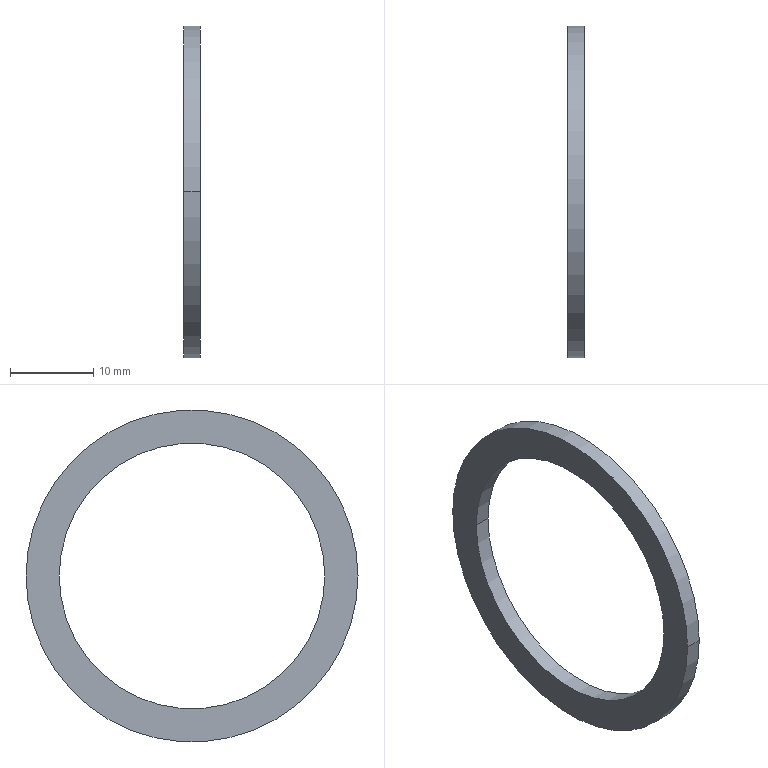Part | NX | features BREP 1 | 1 solid | 6 faces | box 2 x 40 x 40 mm | volume 904.779 mm3 | cylinder 4 | plane 2 | commonest cylinder face diameters 32 x2 40 x2
STEP:
#1=CARTESIAN_POINT('',(-531.355,16.,0.));
#2=VERTEX_POINT('',#1);
#3=CARTESIAN_POINT('',(-531.355,-16.,0.));
#4=VERTEX_POINT('',#3);
#5=CARTESIAN_POINT('',(-531.355,0.,0.));
#6=DIRECTION('',(-1.,0.,0.));
#7=DIRECTION('',(0.,-1.,0.));
#8=AXIS2_PLACEMENT_3D('',#5,#6,#7);
#9=CIRCLE('',#8,16.);
#10=EDGE_CURVE('',#2,#4,#9,.T.);
#11=ORIENTED_EDGE('',*,*,#10,.T.);
#12=CARTESIAN_POINT('',(-529.355,-16.,0.));
#13=VERTEX_POINT('',#12);
#14=CARTESIAN_POINT('',(-531.355,-16.,0.));
#15=DIRECTION('',(1.,0.,0.));
#16=VECTOR('',#15,1000.);
#17=LINE('',#14,#16);
#18=EDGE_CURVE('',#4,#13,#17,.T.);
#19=ORIENTED_EDGE('',*,*,#18,.T.);
#20=CARTESIAN_POINT('',(-529.355,16.,0.));
#21=VERTEX_POINT('',#20);
#22=CARTESIAN_POINT('',(-529.355,0.,0.));
#23=DIRECTION('',(-1.,0.,0.));
#24=DIRECTION('',(0.,-1.,0.));
#25=AXIS2_PLACEMENT_3D('',#22,#23,#24);
#26=CIRCLE('',#25,16.);
#27=EDGE_CURVE('',#21,#13,#26,.T.);
#28=ORIENTED_EDGE('',*,*,#27,.F.);
#29=CARTESIAN_POINT('',(-531.355,16.,0.));
#30=DIRECTION('',(1.,0.,0.));
#31=VECTOR('',#30,1000.);
#32=LINE('',#29,#31);
#33=EDGE_CURVE('',#2,#21,#32,.T.);
#34=ORIENTED_EDGE('',*,*,#33,.F.);
#35=EDGE_LOOP('',(#11,#19,#28,#34));
#36=FACE_BOUND('',#35,.T.);
#37=CARTESIAN_POINT('',(-531.355,0.,0.));
#38=DIRECTION('',(1.,0.,0.));
#39=DIRECTION('',(0.,1.,0.));
#40=AXIS2_PLACEMENT_3D('',#37,#38,#39);
#41=CYLINDRICAL_SURFACE('',#40,16.);
#42=ADVANCED_FACE('',(#36),#41,.F.);
#43=CARTESIAN_POINT('',(-531.355,-20.,0.));
#44=VERTEX_POINT('',#43);
#45=CARTESIAN_POINT('',(-531.355,20.,0.));
#46=VERTEX_POINT('',#45);
#47=CARTESIAN_POINT('',(-531.355,0.,0.));
#48=DIRECTION('',(-1.,0.,0.));
#49=DIRECTION('',(0.,-1.,0.));
#50=AXIS2_PLACEMENT_3D('',#47,#48,#49);
#51=CIRCLE('',#50,20.);
#52=EDGE_CURVE('',#44,#46,#51,.T.);
#53=ORIENTED_EDGE('',*,*,#52,.F.);
#54=CARTESIAN_POINT('',(-529.355,-20.,0.));
#55=VERTEX_POINT('',#54);
#56=CARTESIAN_POINT('',(-531.355,-20.,0.));
#57=DIRECTION('',(1.,0.,0.));
#58=VECTOR('',#57,1000.);
#59=LINE('',#56,#58);
#60=EDGE_CURVE('',#44,#55,#59,.T.);
#61=ORIENTED_EDGE('',*,*,#60,.T.);
#62=CARTESIAN_POINT('',(-529.355,20.,0.));
#63=VERTEX_POINT('',#62);
#64=CARTESIAN_POINT('',(-529.355,0.,0.));
#65=DIRECTION('',(-1.,0.,0.));
#66=DIRECTION('',(0.,-1.,0.));
#67=AXIS2_PLACEMENT_3D('',#64,#65,#66);
#68=CIRCLE('',#67,20.);
#69=EDGE_CURVE('',#55,#63,#68,.T.);
#70=ORIENTED_EDGE('',*,*,#69,.T.);
#71=CARTESIAN_POINT('',(-531.355,20.,0.));
#72=DIRECTION('',(1.,0.,0.));
#73=VECTOR('',#72,1000.);
#74=LINE('',#71,#73);
#75=EDGE_CURVE('',#46,#63,#74,.T.);
#76=ORIENTED_EDGE('',*,*,#75,.F.);
#77=EDGE_LOOP('',(#53,#61,#70,#76));
#78=FACE_BOUND('',#77,.T.);
#79=CARTESIAN_POINT('',(-531.355,0.,0.));
#80=DIRECTION('',(1.,0.,0.));
#81=DIRECTION('',(0.,1.,0.));
#82=AXIS2_PLACEMENT_3D('',#79,#80,#81);
#83=CYLINDRICAL_SURFACE('',#82,20.);
#84=ADVANCED_FACE('',(#78),#83,.T.);
#85=CARTESIAN_POINT('',(-531.355,0.,0.));
#86=DIRECTION('',(-1.,0.,0.));
#87=DIRECTION('',(0.,-1.,0.));
#88=AXIS2_PLACEMENT_3D('',#85,#86,#87);
#89=CIRCLE('',#88,20.);
#90=EDGE_CURVE('',#46,#44,#89,.T.);
#91=ORIENTED_EDGE('',*,*,#90,.T.);
#92=ORIENTED_EDGE('',*,*,#52,.T.);
#93=EDGE_LOOP('',(#91,#92));
#94=FACE_BOUND('',#93,.T.);
#95=ORIENTED_EDGE('',*,*,#10,.F.);
#96=CARTESIAN_POINT('',(-531.355,0.,0.));
#97=DIRECTION('',(-1.,0.,0.));
#98=DIRECTION('',(0.,-1.,0.));
#99=AXIS2_PLACEMENT_3D('',#96,#97,#98);
#100=CIRCLE('',#99,16.);
#101=EDGE_CURVE('',#4,#2,#100,.T.);
#102=ORIENTED_EDGE('',*,*,#101,.F.);
#103=EDGE_LOOP('',(#95,#102));
#104=FACE_BOUND('',#103,.T.);
#105=CARTESIAN_POINT('',(-531.355,0.,0.));
#106=DIRECTION('',(-1.,0.,0.));
#107=DIRECTION('',(0.,-1.,0.));
#108=AXIS2_PLACEMENT_3D('',#105,#106,#107);
#109=PLANE('',#108);
#110=ADVANCED_FACE('',(#94,#104),#109,.T.);
#111=CARTESIAN_POINT('',(-529.355,0.,0.));
#112=DIRECTION('',(-1.,0.,0.));
#113=DIRECTION('',(0.,-1.,0.));
#114=AXIS2_PLACEMENT_3D('',#111,#112,#113);
#115=CIRCLE('',#114,20.);
#116=EDGE_CURVE('',#63,#55,#115,.T.);
#117=ORIENTED_EDGE('',*,*,#116,.F.);
#118=ORIENTED_EDGE('',*,*,#69,.F.);
#119=EDGE_LOOP('',(#117,#118));
#120=FACE_BOUND('',#119,.T.);
#121=ORIENTED_EDGE('',*,*,#27,.T.);
#122=CARTESIAN_POINT('',(-529.355,0.,0.));
#123=DIRECTION('',(-1.,0.,0.));
#124=DIRECTION('',(0.,-1.,0.));
#125=AXIS2_PLACEMENT_3D('',#122,#123,#124);
#126=CIRCLE('',#125,16.);
#127=EDGE_CURVE('',#13,#21,#126,.T.);
#128=ORIENTED_EDGE('',*,*,#127,.T.);
#129=EDGE_LOOP('',(#121,#128));
#130=FACE_BOUND('',#129,.T.);
#131=CARTESIAN_POINT('',(-529.355,0.,0.));
#132=DIRECTION('',(-1.,0.,0.));
#133=DIRECTION('',(0.,-1.,0.));
#134=AXIS2_PLACEMENT_3D('',#131,#132,#133);
#135=PLANE('',#134);
#136=ADVANCED_FACE('',(#120,#130),#135,.F.);
#137=ORIENTED_EDGE('',*,*,#60,.F.);
#138=ORIENTED_EDGE('',*,*,#90,.F.);
#139=ORIENTED_EDGE('',*,*,#75,.T.);
#140=ORIENTED_EDGE('',*,*,#116,.T.);
#141=EDGE_LOOP('',(#137,#138,#139,#140));
#142=FACE_BOUND('',#141,.T.);
#143=CARTESIAN_POINT('',(-531.355,0.,0.));
#144=DIRECTION('',(1.,0.,0.));
#145=DIRECTION('',(0.,1.,0.));
#146=AXIS2_PLACEMENT_3D('',#143,#144,#145);
#147=CYLINDRICAL_SURFACE('',#146,20.);
#148=ADVANCED_FACE('',(#142),#147,.T.);
#149=ORIENTED_EDGE('',*,*,#18,.F.);
#150=ORIENTED_EDGE('',*,*,#101,.T.);
#151=ORIENTED_EDGE('',*,*,#33,.T.);
#152=ORIENTED_EDGE('',*,*,#127,.F.);
#153=EDGE_LOOP('',(#149,#150,#151,#152));
#154=FACE_BOUND('',#153,.T.);
#155=CARTESIAN_POINT('',(-531.355,0.,0.));
#156=DIRECTION('',(1.,0.,0.));
#157=DIRECTION('',(0.,1.,0.));
#158=AXIS2_PLACEMENT_3D('',#155,#156,#157);
#159=CYLINDRICAL_SURFACE('',#158,16.);
#160=ADVANCED_FACE('',(#154),#159,.F.);
#161=CLOSED_SHELL('',(#42,#84,#110,#136,#148,#160));
#162=MANIFOLD_SOLID_BREP('',#161);
#163=(LENGTH_UNIT()NAMED_UNIT(*)SI_UNIT(.MILLI.,.METRE.));
#164=UNCERTAINTY_MEASURE_WITH_UNIT(LENGTH_MEASURE(0.00001),#163,'','');
#165=(NAMED_UNIT(*)PLANE_ANGLE_UNIT()SI_UNIT($,.RADIAN.));
#166=(NAMED_UNIT(*)SI_UNIT($,.STERADIAN.)SOLID_ANGLE_UNIT());
#167=(GEOMETRIC_REPRESENTATION_CONTEXT(3)GLOBAL_UNCERTAINTY_ASSIGNED_CONTEXT((#164))GLOBAL_UNIT_ASSIGNED_CONTEXT((#163,#165,#166))REPRESENTATION_CONTEXT('',''));
#168=ADVANCED_BREP_SHAPE_REPRESENTATION('',(#162),#167);